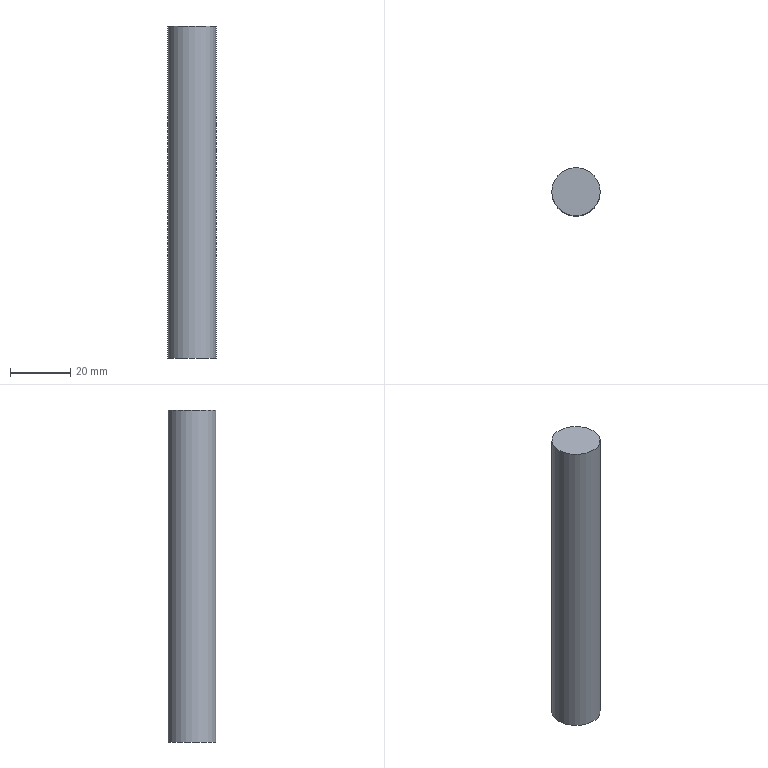Part | STEP file | solid 216 | 1 solid | 3 faces | box 16 x 16 x 110 mm | volume 22117 mm3 | plane 2 | cylinder 1 | commonest cylinder face diameters 16 x1